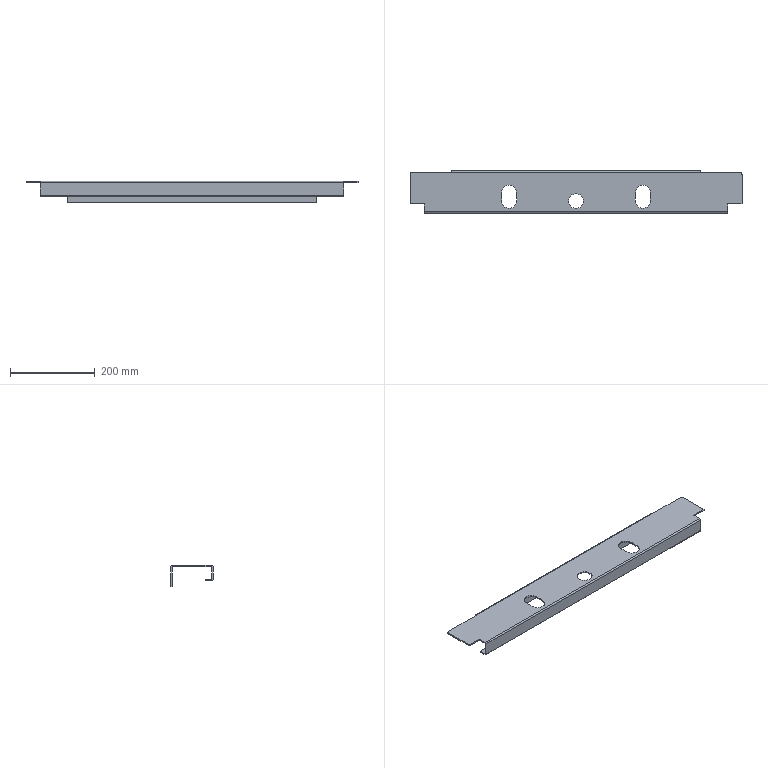Part | STEP file | HESS-408-70-15W-W-15-bottom frame 5 | 1 solid | 47 faces | box 785 x 100 x 50 mm | volume 395842 mm3 | plane 27 | cylinder 20 | commonest cylinder face diameters 35 x6 40 x6 0.2 x3 6.2 x3 10 x2